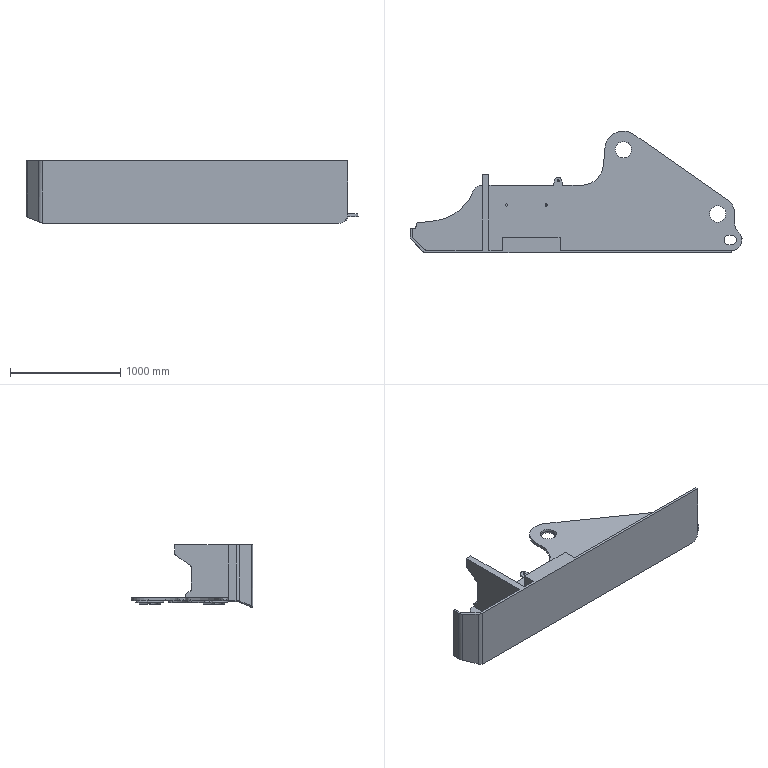Part | NX | features 底座(默认<按焊接>) 2 | 1 solid | 120 faces | box 3009 x 1102 x 567 mm | volume 135543302 mm3 | plane 79 | cylinder 40 | sphere 1 | commonest cylinder face diameters 100 x5 40 x4 56.36 x4 251 x4 20 x3 87.28 x2